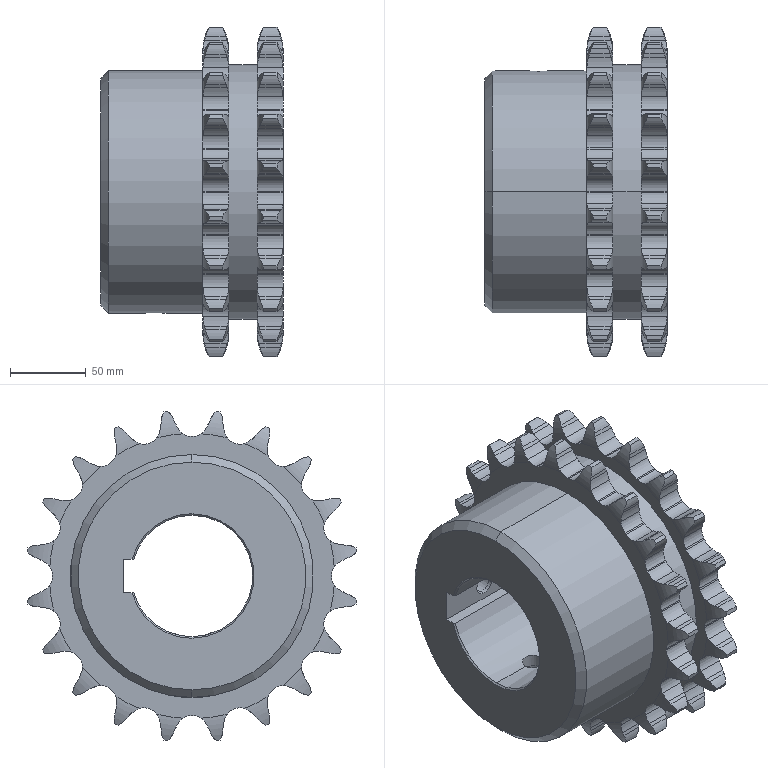Part | STEP file | Input 110 | 1 solid | 533 faces | box 120 x 217.216 x 217.216 mm | volume 2149688 mm3 | cylinder 311 | plane 130 | torus 80 | cone 8 | spline 4 | commonest cylinder face diameters 19.221 x88 31.513 x84 49.701 x84 219.512 x40 14 x4 16 x4